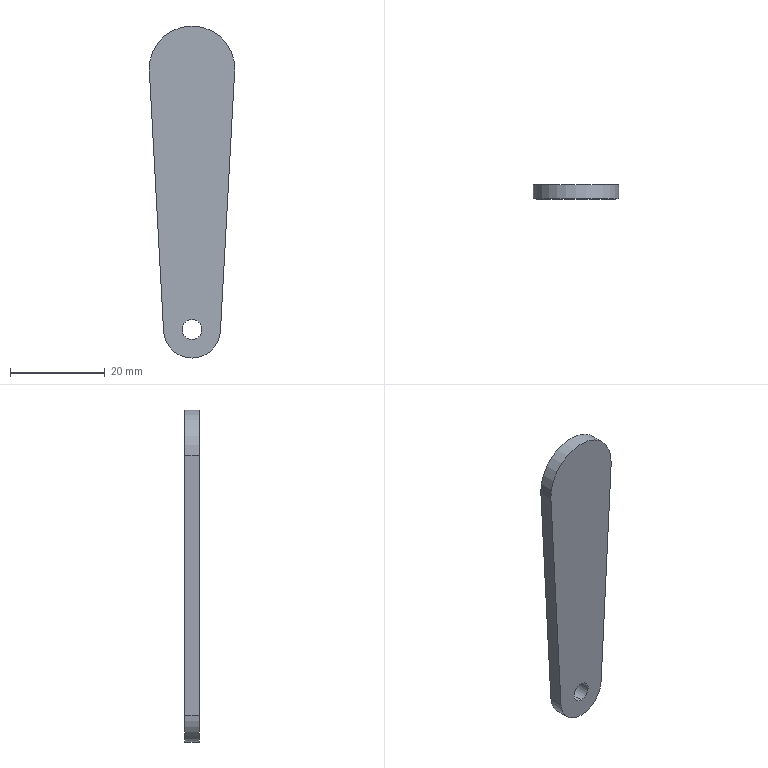Part | STEP file | Handwheel sub-plate | 1 solid | 9 faces | box 18 x 3 x 70 mm | volume 2988 mm3 | cylinder 5 | plane 4 | commonest cylinder face diameters 4.2 x2 12 x2 18 x1
STEP:
#1=CARTESIAN_POINT('',(0.,0.,0.));
#2=DIRECTION('',(0.,0.,1.));
#3=DIRECTION('',(1.,0.,0.));
#4=AXIS2_PLACEMENT_3D('',#1,#2,#3);
#5=CARTESIAN_POINT('',(0.,-1.5,2.1));
#6=VERTEX_POINT('',#5);
#7=CARTESIAN_POINT('',(0.,1.5,2.1));
#8=VERTEX_POINT('',#7);
#9=CARTESIAN_POINT('',(0.,1.5,2.1));
#10=DIRECTION('',(0.,1.,0.));
#11=VECTOR('',#10,1.);
#12=LINE('',#9,#11);
#13=CARTESIAN_POINT('',(0.,1.5,0.));
#14=DIRECTION('',(0.,1.,0.));
#15=DIRECTION('',(0.,0.,1.));
#16=AXIS2_PLACEMENT_3D('',#13,#14,#15);
#17=CYLINDRICAL_SURFACE('',#16,2.1);
#18=CARTESIAN_POINT('',(6.283,0.));
#19=DIRECTION('',(0.,1.));
#20=VECTOR('',#19,1.);
#21=LINE('',#18,#20);
#22=(GEOMETRIC_REPRESENTATION_CONTEXT(2)PARAMETRIC_REPRESENTATION_CONTEXT()REPRESENTATION_CONTEXT('',''));
#23=DEFINITIONAL_REPRESENTATION('',(#21),#22);
#24=PCURVE('',#17,#23);
#25=CARTESIAN_POINT('',(0.,1.5,0.));
#26=DIRECTION('',(0.,1.,0.));
#27=DIRECTION('',(0.,0.,1.));
#28=AXIS2_PLACEMENT_3D('',#25,#26,#27);
#29=CYLINDRICAL_SURFACE('',#28,2.1);
#30=CARTESIAN_POINT('',(0.,0.));
#31=DIRECTION('',(0.,1.));
#32=VECTOR('',#31,1.);
#33=LINE('',#30,#32);
#34=(GEOMETRIC_REPRESENTATION_CONTEXT(2)PARAMETRIC_REPRESENTATION_CONTEXT()REPRESENTATION_CONTEXT('',''));
#35=DEFINITIONAL_REPRESENTATION('',(#33),#34);
#36=PCURVE('',#29,#35);
#37=SURFACE_CURVE('',#12,(#24,#36),.PCURVE_S1.);
#38=EDGE_CURVE('',#6,#8,#37,.T.);
#39=ORIENTED_EDGE('',*,*,#38,.T.);
#40=CARTESIAN_POINT('',(0.,1.5,-2.1));
#41=VERTEX_POINT('',#40);
#42=CARTESIAN_POINT('',(0.,1.5,0.));
#43=DIRECTION('',(0.,1.,0.));
#44=DIRECTION('',(0.,0.,1.));
#45=AXIS2_PLACEMENT_3D('',#42,#43,#44);
#46=CIRCLE('',#45,2.1);
#47=CARTESIAN_POINT('',(0.,0.));
#48=DIRECTION('',(1.,0.));
#49=VECTOR('',#48,1.);
#50=LINE('',#47,#49);
#51=(GEOMETRIC_REPRESENTATION_CONTEXT(2)PARAMETRIC_REPRESENTATION_CONTEXT()REPRESENTATION_CONTEXT('',''));
#52=DEFINITIONAL_REPRESENTATION('',(#50),#51);
#53=PCURVE('',#17,#52);
#54=CARTESIAN_POINT('',(0.,1.5,0.));
#55=DIRECTION('',(0.,1.,0.));
#56=DIRECTION('',(0.,0.,1.));
#57=AXIS2_PLACEMENT_3D('',#54,#55,#56);
#58=PLANE('',#57);
#59=CARTESIAN_POINT('',(0.,0.));
#60=DIRECTION('',(1.,0.));
#61=AXIS2_PLACEMENT_2D('',#59,#60);
#62=CIRCLE('',#61,2.1);
#63=(GEOMETRIC_REPRESENTATION_CONTEXT(2)PARAMETRIC_REPRESENTATION_CONTEXT()REPRESENTATION_CONTEXT('',''));
#64=DEFINITIONAL_REPRESENTATION('',(#62),#63);
#65=PCURVE('',#58,#64);
#66=SURFACE_CURVE('',#46,(#53,#65),.PCURVE_S1.);
#67=EDGE_CURVE('',#41,#8,#66,.T.);
#68=ORIENTED_EDGE('',*,*,#67,.F.);
#69=CARTESIAN_POINT('',(0.,-1.5,-2.1));
#70=VERTEX_POINT('',#69);
#71=CARTESIAN_POINT('',(0.,1.5,-2.1));
#72=DIRECTION('',(0.,1.,0.));
#73=VECTOR('',#72,1.);
#74=LINE('',#71,#73);
#75=CARTESIAN_POINT('',(3.142,0.));
#76=DIRECTION('',(0.,1.));
#77=VECTOR('',#76,1.);
#78=LINE('',#75,#77);
#79=(GEOMETRIC_REPRESENTATION_CONTEXT(2)PARAMETRIC_REPRESENTATION_CONTEXT()REPRESENTATION_CONTEXT('',''));
#80=DEFINITIONAL_REPRESENTATION('',(#78),#79);
#81=PCURVE('',#17,#80);
#82=CARTESIAN_POINT('',(3.142,0.));
#83=DIRECTION('',(0.,1.));
#84=VECTOR('',#83,1.);
#85=LINE('',#82,#84);
#86=(GEOMETRIC_REPRESENTATION_CONTEXT(2)PARAMETRIC_REPRESENTATION_CONTEXT()REPRESENTATION_CONTEXT('',''));
#87=DEFINITIONAL_REPRESENTATION('',(#85),#86);
#88=PCURVE('',#29,#87);
#89=SURFACE_CURVE('',#74,(#81,#88),.PCURVE_S1.);
#90=EDGE_CURVE('',#70,#41,#89,.T.);
#91=ORIENTED_EDGE('',*,*,#90,.F.);
#92=CARTESIAN_POINT('',(0.,-1.5,0.));
#93=DIRECTION('',(0.,1.,0.));
#94=DIRECTION('',(0.,0.,1.));
#95=AXIS2_PLACEMENT_3D('',#92,#93,#94);
#96=CIRCLE('',#95,2.1);
#97=CARTESIAN_POINT('',(0.,-3.));
#98=DIRECTION('',(1.,0.));
#99=VECTOR('',#98,1.);
#100=LINE('',#97,#99);
#101=(GEOMETRIC_REPRESENTATION_CONTEXT(2)PARAMETRIC_REPRESENTATION_CONTEXT()REPRESENTATION_CONTEXT('',''));
#102=DEFINITIONAL_REPRESENTATION('',(#100),#101);
#103=PCURVE('',#17,#102);
#104=CARTESIAN_POINT('',(0.,-1.5,0.));
#105=DIRECTION('',(0.,1.,0.));
#106=DIRECTION('',(0.,0.,1.));
#107=AXIS2_PLACEMENT_3D('',#104,#105,#106);
#108=PLANE('',#107);
#109=CARTESIAN_POINT('',(0.,0.));
#110=DIRECTION('',(1.,0.));
#111=AXIS2_PLACEMENT_2D('',#109,#110);
#112=CIRCLE('',#111,2.1);
#113=(GEOMETRIC_REPRESENTATION_CONTEXT(2)PARAMETRIC_REPRESENTATION_CONTEXT()REPRESENTATION_CONTEXT('',''));
#114=DEFINITIONAL_REPRESENTATION('',(#112),#113);
#115=PCURVE('',#108,#114);
#116=SURFACE_CURVE('',#96,(#103,#115),.PCURVE_S1.);
#117=EDGE_CURVE('',#70,#6,#116,.T.);
#118=ORIENTED_EDGE('',*,*,#117,.T.);
#119=EDGE_LOOP('',(#39,#68,#91,#118));
#120=FACE_BOUND('',#119,.F.);
#121=ADVANCED_FACE('',(#120),#17,.F.);
#122=CARTESIAN_POINT('',(0.,1.5,-6.));
#123=VERTEX_POINT('',#122);
#124=CARTESIAN_POINT('',(-5.991,1.5,-0.3273));
#125=VERTEX_POINT('',#124);
#126=CARTESIAN_POINT('',(0.,1.5,0.));
#127=DIRECTION('',(0.,1.,0.));
#128=DIRECTION('',(0.,0.,1.));
#129=AXIS2_PLACEMENT_3D('',#126,#127,#128);
#130=CIRCLE('',#129,6.);
#131=CARTESIAN_POINT('',(0.,1.5,0.));
#132=DIRECTION('',(0.,-1.,0.));
#133=DIRECTION('',(0.,0.,-1.));
#134=AXIS2_PLACEMENT_3D('',#131,#132,#133);
#135=CYLINDRICAL_SURFACE('',#134,6.);
#136=CARTESIAN_POINT('',(9.425,0.));
#137=DIRECTION('',(-1.,0.));
#138=VECTOR('',#137,1.);
#139=LINE('',#136,#138);
#140=(GEOMETRIC_REPRESENTATION_CONTEXT(2)PARAMETRIC_REPRESENTATION_CONTEXT()REPRESENTATION_CONTEXT('',''));
#141=DEFINITIONAL_REPRESENTATION('',(#139),#140);
#142=PCURVE('',#135,#141);
#143=CARTESIAN_POINT('',(0.,0.));
#144=DIRECTION('',(1.,0.));
#145=AXIS2_PLACEMENT_2D('',#143,#144);
#146=CIRCLE('',#145,6.);
#147=(GEOMETRIC_REPRESENTATION_CONTEXT(2)PARAMETRIC_REPRESENTATION_CONTEXT()REPRESENTATION_CONTEXT('',''));
#148=DEFINITIONAL_REPRESENTATION('',(#146),#147);
#149=PCURVE('',#58,#148);
#150=SURFACE_CURVE('',#130,(#142,#149),.PCURVE_S1.);
#151=EDGE_CURVE('',#123,#125,#150,.T.);
#152=ORIENTED_EDGE('',*,*,#151,.F.);
#153=CARTESIAN_POINT('',(0.,-1.5,-6.));
#154=VERTEX_POINT('',#153);
#155=CARTESIAN_POINT('',(0.,1.5,-6.));
#156=DIRECTION('',(0.,-1.,0.));
#157=VECTOR('',#156,1.);
#158=LINE('',#155,#157);
#159=CARTESIAN_POINT('',(6.283,0.));
#160=DIRECTION('',(0.,1.));
#161=VECTOR('',#160,1.);
#162=LINE('',#159,#161);
#163=(GEOMETRIC_REPRESENTATION_CONTEXT(2)PARAMETRIC_REPRESENTATION_CONTEXT()REPRESENTATION_CONTEXT('',''));
#164=DEFINITIONAL_REPRESENTATION('',(#162),#163);
#165=PCURVE('',#135,#164);
#166=CARTESIAN_POINT('',(0.,1.5,0.));
#167=DIRECTION('',(0.,-1.,0.));
#168=DIRECTION('',(0.,0.,-1.));
#169=AXIS2_PLACEMENT_3D('',#166,#167,#168);
#170=CYLINDRICAL_SURFACE('',#169,6.);
#171=CARTESIAN_POINT('',(0.,0.));
#172=DIRECTION('',(0.,1.));
#173=VECTOR('',#172,1.);
#174=LINE('',#171,#173);
#175=(GEOMETRIC_REPRESENTATION_CONTEXT(2)PARAMETRIC_REPRESENTATION_CONTEXT()REPRESENTATION_CONTEXT('',''));
#176=DEFINITIONAL_REPRESENTATION('',(#174),#175);
#177=PCURVE('',#170,#176);
#178=SURFACE_CURVE('',#158,(#165,#177),.PCURVE_S1.);
#179=EDGE_CURVE('',#123,#154,#178,.T.);
#180=ORIENTED_EDGE('',*,*,#179,.T.);
#181=CARTESIAN_POINT('',(-5.991,-1.5,-0.3273));
#182=VERTEX_POINT('',#181);
#183=CARTESIAN_POINT('',(0.,-1.5,0.));
#184=DIRECTION('',(0.,1.,0.));
#185=DIRECTION('',(0.,0.,1.));
#186=AXIS2_PLACEMENT_3D('',#183,#184,#185);
#187=CIRCLE('',#186,6.);
#188=CARTESIAN_POINT('',(9.425,3.));
#189=DIRECTION('',(-1.,0.));
#190=VECTOR('',#189,1.);
#191=LINE('',#188,#190);
#192=(GEOMETRIC_REPRESENTATION_CONTEXT(2)PARAMETRIC_REPRESENTATION_CONTEXT()REPRESENTATION_CONTEXT('',''));
#193=DEFINITIONAL_REPRESENTATION('',(#191),#192);
#194=PCURVE('',#135,#193);
#195=CARTESIAN_POINT('',(0.,0.));
#196=DIRECTION('',(1.,0.));
#197=AXIS2_PLACEMENT_2D('',#195,#196);
#198=CIRCLE('',#197,6.);
#199=(GEOMETRIC_REPRESENTATION_CONTEXT(2)PARAMETRIC_REPRESENTATION_CONTEXT()REPRESENTATION_CONTEXT('',''));
#200=DEFINITIONAL_REPRESENTATION('',(#198),#199);
#201=PCURVE('',#108,#200);
#202=SURFACE_CURVE('',#187,(#194,#201),.PCURVE_S1.);
#203=EDGE_CURVE('',#154,#182,#202,.T.);
#204=ORIENTED_EDGE('',*,*,#203,.T.);
#205=CARTESIAN_POINT('',(-5.991,1.5,-0.3273));
#206=DIRECTION('',(0.,-1.,0.));
#207=VECTOR('',#206,1.);
#208=LINE('',#205,#207);
#209=CARTESIAN_POINT('',(4.767,0.));
#210=DIRECTION('',(0.,1.));
#211=VECTOR('',#210,1.);
#212=LINE('',#209,#211);
#213=(GEOMETRIC_REPRESENTATION_CONTEXT(2)PARAMETRIC_REPRESENTATION_CONTEXT()REPRESENTATION_CONTEXT('',''));
#214=DEFINITIONAL_REPRESENTATION('',(#212),#213);
#215=PCURVE('',#135,#214);
#216=CARTESIAN_POINT('',(-5.991,1.5,-0.3273));
#217=DIRECTION('',(0.9985,0.,0.05455));
#218=DIRECTION('',(0.05455,0.,-0.9985));
#219=AXIS2_PLACEMENT_3D('',#216,#217,#218);
#220=PLANE('',#219);
#221=CARTESIAN_POINT('',(0.,0.));
#222=DIRECTION('',(0.,-1.));
#223=VECTOR('',#222,1.);
#224=LINE('',#221,#223);
#225=(GEOMETRIC_REPRESENTATION_CONTEXT(2)PARAMETRIC_REPRESENTATION_CONTEXT()REPRESENTATION_CONTEXT('',''));
#226=DEFINITIONAL_REPRESENTATION('',(#224),#225);
#227=PCURVE('',#220,#226);
#228=SURFACE_CURVE('',#208,(#215,#227),.PCURVE_S1.);
#229=EDGE_CURVE('',#125,#182,#228,.T.);
#230=ORIENTED_EDGE('',*,*,#229,.F.);
#231=EDGE_LOOP('',(#152,#180,#204,#230));
#232=FACE_BOUND('',#231,.T.);
#233=ADVANCED_FACE('',(#232),#135,.T.);
#234=ORIENTED_EDGE('',*,*,#179,.F.);
#235=CARTESIAN_POINT('',(5.991,1.5,-0.3273));
#236=VERTEX_POINT('',#235);
#237=CARTESIAN_POINT('',(0.,1.5,0.));
#238=DIRECTION('',(0.,1.,0.));
#239=DIRECTION('',(0.,0.,1.));
#240=AXIS2_PLACEMENT_3D('',#237,#238,#239);
#241=CIRCLE('',#240,6.);
#242=CARTESIAN_POINT('',(3.142,0.));
#243=DIRECTION('',(-1.,0.));
#244=VECTOR('',#243,1.);
#245=LINE('',#242,#244);
#246=(GEOMETRIC_REPRESENTATION_CONTEXT(2)PARAMETRIC_REPRESENTATION_CONTEXT()REPRESENTATION_CONTEXT('',''));
#247=DEFINITIONAL_REPRESENTATION('',(#245),#246);
#248=PCURVE('',#170,#247);
#249=CARTESIAN_POINT('',(0.,0.));
#250=DIRECTION('',(1.,0.));
#251=AXIS2_PLACEMENT_2D('',#249,#250);
#252=CIRCLE('',#251,6.);
#253=(GEOMETRIC_REPRESENTATION_CONTEXT(2)PARAMETRIC_REPRESENTATION_CONTEXT()REPRESENTATION_CONTEXT('',''));
#254=DEFINITIONAL_REPRESENTATION('',(#252),#253);
#255=PCURVE('',#58,#254);
#256=SURFACE_CURVE('',#241,(#248,#255),.PCURVE_S1.);
#257=EDGE_CURVE('',#236,#123,#256,.T.);
#258=ORIENTED_EDGE('',*,*,#257,.F.);
#259=CARTESIAN_POINT('',(5.991,-1.5,-0.3273));
#260=VERTEX_POINT('',#259);
#261=CARTESIAN_POINT('',(5.991,1.5,-0.3273));
#262=DIRECTION('',(0.,-1.,0.));
#263=VECTOR('',#262,1.);
#264=LINE('',#261,#263);
#265=CARTESIAN_POINT('',(1.516,0.));
#266=DIRECTION('',(0.,1.));
#267=VECTOR('',#266,1.);
#268=LINE('',#265,#267);
#269=(GEOMETRIC_REPRESENTATION_CONTEXT(2)PARAMETRIC_REPRESENTATION_CONTEXT()REPRESENTATION_CONTEXT('',''));
#270=DEFINITIONAL_REPRESENTATION('',(#268),#269);
#271=PCURVE('',#170,#270);
#272=CARTESIAN_POINT('',(8.987,1.5,54.509));
#273=DIRECTION('',(-0.9985,0.,0.05455));
#274=DIRECTION('',(0.05455,0.,0.9985));
#275=AXIS2_PLACEMENT_3D('',#272,#273,#274);
#276=PLANE('',#275);
#277=CARTESIAN_POINT('',(-54.918,0.));
#278=DIRECTION('',(0.,-1.));
#279=VECTOR('',#278,1.);
#280=LINE('',#277,#279);
#281=(GEOMETRIC_REPRESENTATION_CONTEXT(2)PARAMETRIC_REPRESENTATION_CONTEXT()REPRESENTATION_CONTEXT('',''));
#282=DEFINITIONAL_REPRESENTATION('',(#280),#281);
#283=PCURVE('',#276,#282);
#284=SURFACE_CURVE('',#264,(#271,#283),.PCURVE_S1.);
#285=EDGE_CURVE('',#236,#260,#284,.T.);
#286=ORIENTED_EDGE('',*,*,#285,.T.);
#287=CARTESIAN_POINT('',(0.,-1.5,0.));
#288=DIRECTION('',(0.,1.,0.));
#289=DIRECTION('',(0.,0.,1.));
#290=AXIS2_PLACEMENT_3D('',#287,#288,#289);
#291=CIRCLE('',#290,6.);
#292=CARTESIAN_POINT('',(3.142,3.));
#293=DIRECTION('',(-1.,0.));
#294=VECTOR('',#293,1.);
#295=LINE('',#292,#294);
#296=(GEOMETRIC_REPRESENTATION_CONTEXT(2)PARAMETRIC_REPRESENTATION_CONTEXT()REPRESENTATION_CONTEXT('',''));
#297=DEFINITIONAL_REPRESENTATION('',(#295),#296);
#298=PCURVE('',#170,#297);
#299=CARTESIAN_POINT('',(0.,0.));
#300=DIRECTION('',(1.,0.));
#301=AXIS2_PLACEMENT_2D('',#299,#300);
#302=CIRCLE('',#301,6.);
#303=(GEOMETRIC_REPRESENTATION_CONTEXT(2)PARAMETRIC_REPRESENTATION_CONTEXT()REPRESENTATION_CONTEXT('',''));
#304=DEFINITIONAL_REPRESENTATION('',(#302),#303);
#305=PCURVE('',#108,#304);
#306=SURFACE_CURVE('',#291,(#298,#305),.PCURVE_S1.);
#307=EDGE_CURVE('',#260,#154,#306,.T.);
#308=ORIENTED_EDGE('',*,*,#307,.T.);
#309=EDGE_LOOP('',(#234,#258,#286,#308));
#310=FACE_BOUND('',#309,.T.);
#311=ADVANCED_FACE('',(#310),#170,.T.);
#312=CARTESIAN_POINT('',(-8.987,-1.5,54.509));
#313=VERTEX_POINT('',#312);
#314=CARTESIAN_POINT('',(-5.991,-1.5,-0.3273));
#315=DIRECTION('',(-0.05455,0.,0.9985));
#316=VECTOR('',#315,1.);
#317=LINE('',#314,#316);
#318=CARTESIAN_POINT('',(0.,-3.));
#319=DIRECTION('',(-1.,0.));
#320=VECTOR('',#319,1.);
#321=LINE('',#318,#320);
#322=(GEOMETRIC_REPRESENTATION_CONTEXT(2)PARAMETRIC_REPRESENTATION_CONTEXT()REPRESENTATION_CONTEXT('',''));
#323=DEFINITIONAL_REPRESENTATION('',(#321),#322);
#324=PCURVE('',#220,#323);
#325=CARTESIAN_POINT('',(-0.3273,-5.991));
#326=DIRECTION('',(0.9985,-0.05455));
#327=VECTOR('',#326,1.);
#328=LINE('',#325,#327);
#329=(GEOMETRIC_REPRESENTATION_CONTEXT(2)PARAMETRIC_REPRESENTATION_CONTEXT()REPRESENTATION_CONTEXT('',''));
#330=DEFINITIONAL_REPRESENTATION('',(#328),#329);
#331=PCURVE('',#108,#330);
#332=SURFACE_CURVE('',#317,(#324,#331),.PCURVE_S1.);
#333=EDGE_CURVE('',#182,#313,#332,.T.);
#334=ORIENTED_EDGE('',*,*,#333,.T.);
#335=CARTESIAN_POINT('',(-8.987,1.5,54.509));
#336=VERTEX_POINT('',#335);
#337=CARTESIAN_POINT('',(-8.987,1.5,54.509));
#338=DIRECTION('',(0.,-1.,0.));
#339=VECTOR('',#338,1.);
#340=LINE('',#337,#339);
#341=CARTESIAN_POINT('',(-54.918,0.));
#342=DIRECTION('',(0.,-1.));
#343=VECTOR('',#342,1.);
#344=LINE('',#341,#343);
#345=(GEOMETRIC_REPRESENTATION_CONTEXT(2)PARAMETRIC_REPRESENTATION_CONTEXT()REPRESENTATION_CONTEXT('',''));
#346=DEFINITIONAL_REPRESENTATION('',(#344),#345);
#347=PCURVE('',#220,#346);
#348=CARTESIAN_POINT('',(0.,1.5,55.));
#349=DIRECTION('',(0.,-1.,0.));
#350=DIRECTION('',(0.,0.,-1.));
#351=AXIS2_PLACEMENT_3D('',#348,#349,#350);
#352=CYLINDRICAL_SURFACE('',#351,9.);
#353=CARTESIAN_POINT('',(4.767,0.));
#354=DIRECTION('',(0.,1.));
#355=VECTOR('',#354,1.);
#356=LINE('',#353,#355);
#357=(GEOMETRIC_REPRESENTATION_CONTEXT(2)PARAMETRIC_REPRESENTATION_CONTEXT()REPRESENTATION_CONTEXT('',''));
#358=DEFINITIONAL_REPRESENTATION('',(#356),#357);
#359=PCURVE('',#352,#358);
#360=SURFACE_CURVE('',#340,(#347,#359),.PCURVE_S1.);
#361=EDGE_CURVE('',#336,#313,#360,.T.);
#362=ORIENTED_EDGE('',*,*,#361,.F.);
#363=CARTESIAN_POINT('',(-5.991,1.5,-0.3273));
#364=DIRECTION('',(-0.05455,0.,0.9985));
#365=VECTOR('',#364,1.);
#366=LINE('',#363,#365);
#367=CARTESIAN_POINT('',(0.,0.));
#368=DIRECTION('',(-1.,0.));
#369=VECTOR('',#368,1.);
#370=LINE('',#367,#369);
#371=(GEOMETRIC_REPRESENTATION_CONTEXT(2)PARAMETRIC_REPRESENTATION_CONTEXT()REPRESENTATION_CONTEXT('',''));
#372=DEFINITIONAL_REPRESENTATION('',(#370),#371);
#373=PCURVE('',#220,#372);
#374=CARTESIAN_POINT('',(-0.3273,-5.991));
#375=DIRECTION('',(0.9985,-0.05455));
#376=VECTOR('',#375,1.);
#377=LINE('',#374,#376);
#378=(GEOMETRIC_REPRESENTATION_CONTEXT(2)PARAMETRIC_REPRESENTATION_CONTEXT()REPRESENTATION_CONTEXT('',''));
#379=DEFINITIONAL_REPRESENTATION('',(#377),#378);
#380=PCURVE('',#58,#379);
#381=SURFACE_CURVE('',#366,(#373,#380),.PCURVE_S1.);
#382=EDGE_CURVE('',#125,#336,#381,.T.);
#383=ORIENTED_EDGE('',*,*,#382,.F.);
#384=ORIENTED_EDGE('',*,*,#229,.T.);
#385=EDGE_LOOP('',(#334,#362,#383,#384));
#386=FACE_BOUND('',#385,.T.);
#387=ADVANCED_FACE('',(#386),#220,.F.);
#388=CARTESIAN_POINT('',(8.987,-1.5,54.509));
#389=VERTEX_POINT('',#388);
#390=CARTESIAN_POINT('',(0.,-1.5,55.));
#391=DIRECTION('',(0.,1.,0.));
#392=DIRECTION('',(0.,0.,1.));
#393=AXIS2_PLACEMENT_3D('',#390,#391,#392);
#394=CIRCLE('',#393,9.);
#395=CARTESIAN_POINT('',(9.425,3.));
#396=DIRECTION('',(-1.,0.));
#397=VECTOR('',#396,1.);
#398=LINE('',#395,#397);
#399=(GEOMETRIC_REPRESENTATION_CONTEXT(2)PARAMETRIC_REPRESENTATION_CONTEXT()REPRESENTATION_CONTEXT('',''));
#400=DEFINITIONAL_REPRESENTATION('',(#398),#399);
#401=PCURVE('',#352,#400);
#402=CARTESIAN_POINT('',(55.,0.));
#403=DIRECTION('',(1.,0.));
#404=AXIS2_PLACEMENT_2D('',#402,#403);
#405=CIRCLE('',#404,9.);
#406=(GEOMETRIC_REPRESENTATION_CONTEXT(2)PARAMETRIC_REPRESENTATION_CONTEXT()REPRESENTATION_CONTEXT('',''));
#407=DEFINITIONAL_REPRESENTATION('',(#405),#406);
#408=PCURVE('',#108,#407);
#409=SURFACE_CURVE('',#394,(#401,#408),.PCURVE_S1.);
#410=EDGE_CURVE('',#313,#389,#409,.T.);
#411=ORIENTED_EDGE('',*,*,#410,.T.);
#412=CARTESIAN_POINT('',(8.987,1.5,54.509));
#413=VERTEX_POINT('',#412);
#414=CARTESIAN_POINT('',(8.987,1.5,54.509));
#415=DIRECTION('',(0.,-1.,0.));
#416=VECTOR('',#415,1.);
#417=LINE('',#414,#416);
#418=CARTESIAN_POINT('',(1.516,0.));
#419=DIRECTION('',(0.,1.));
#420=VECTOR('',#419,1.);
#421=LINE('',#418,#420);
#422=(GEOMETRIC_REPRESENTATION_CONTEXT(2)PARAMETRIC_REPRESENTATION_CONTEXT()REPRESENTATION_CONTEXT('',''));
#423=DEFINITIONAL_REPRESENTATION('',(#421),#422);
#424=PCURVE('',#352,#423);
#425=CARTESIAN_POINT('',(0.,0.));
#426=DIRECTION('',(0.,-1.));
#427=VECTOR('',#426,1.);
#428=LINE('',#425,#427);
#429=(GEOMETRIC_REPRESENTATION_CONTEXT(2)PARAMETRIC_REPRESENTATION_CONTEXT()REPRESENTATION_CONTEXT('',''));
#430=DEFINITIONAL_REPRESENTATION('',(#428),#429);
#431=PCURVE('',#276,#430);
#432=SURFACE_CURVE('',#417,(#424,#431),.PCURVE_S1.);
#433=EDGE_CURVE('',#413,#389,#432,.T.);
#434=ORIENTED_EDGE('',*,*,#433,.F.);
#435=CARTESIAN_POINT('',(0.,1.5,55.));
#436=DIRECTION('',(0.,1.,0.));
#437=DIRECTION('',(0.,0.,1.));
#438=AXIS2_PLACEMENT_3D('',#435,#436,#437);
#439=CIRCLE('',#438,9.);
#440=CARTESIAN_POINT('',(9.425,0.));
#441=DIRECTION('',(-1.,0.));
#442=VECTOR('',#441,1.);
#443=LINE('',#440,#442);
#444=(GEOMETRIC_REPRESENTATION_CONTEXT(2)PARAMETRIC_REPRESENTATION_CONTEXT()REPRESENTATION_CONTEXT('',''));
#445=DEFINITIONAL_REPRESENTATION('',(#443),#444);
#446=PCURVE('',#352,#445);
#447=CARTESIAN_POINT('',(55.,0.));
#448=DIRECTION('',(1.,0.));
#449=AXIS2_PLACEMENT_2D('',#447,#448);
#450=CIRCLE('',#449,9.);
#451=(GEOMETRIC_REPRESENTATION_CONTEXT(2)PARAMETRIC_REPRESENTATION_CONTEXT()REPRESENTATION_CONTEXT('',''));
#452=DEFINITIONAL_REPRESENTATION('',(#450),#451);
#453=PCURVE('',#58,#452);
#454=SURFACE_CURVE('',#439,(#446,#453),.PCURVE_S1.);
#455=EDGE_CURVE('',#336,#413,#454,.T.);
#456=ORIENTED_EDGE('',*,*,#455,.F.);
#457=ORIENTED_EDGE('',*,*,#361,.T.);
#458=EDGE_LOOP('',(#411,#434,#456,#457));
#459=FACE_BOUND('',#458,.T.);
#460=ADVANCED_FACE('',(#459),#352,.T.);
#461=CARTESIAN_POINT('',(8.987,-1.5,54.509));
#462=DIRECTION('',(-0.05455,0.,-0.9985));
#463=VECTOR('',#462,1.);
#464=LINE('',#461,#463);
#465=CARTESIAN_POINT('',(0.,-3.));
#466=DIRECTION('',(-1.,0.));
#467=VECTOR('',#466,1.);
#468=LINE('',#465,#467);
#469=(GEOMETRIC_REPRESENTATION_CONTEXT(2)PARAMETRIC_REPRESENTATION_CONTEXT()REPRESENTATION_CONTEXT('',''));
#470=DEFINITIONAL_REPRESENTATION('',(#468),#469);
#471=PCURVE('',#276,#470);
#472=CARTESIAN_POINT('',(54.509,8.987));
#473=DIRECTION('',(-0.9985,-0.05455));
#474=VECTOR('',#473,1.);
#475=LINE('',#472,#474);
#476=(GEOMETRIC_REPRESENTATION_CONTEXT(2)PARAMETRIC_REPRESENTATION_CONTEXT()REPRESENTATION_CONTEXT('',''));
#477=DEFINITIONAL_REPRESENTATION('',(#475),#476);
#478=PCURVE('',#108,#477);
#479=SURFACE_CURVE('',#464,(#471,#478),.PCURVE_S1.);
#480=EDGE_CURVE('',#389,#260,#479,.T.);
#481=ORIENTED_EDGE('',*,*,#480,.T.);
#482=ORIENTED_EDGE('',*,*,#285,.F.);
#483=CARTESIAN_POINT('',(8.987,1.5,54.509));
#484=DIRECTION('',(-0.05455,0.,-0.9985));
#485=VECTOR('',#484,1.);
#486=LINE('',#483,#485);
#487=CARTESIAN_POINT('',(0.,0.));
#488=DIRECTION('',(-1.,0.));
#489=VECTOR('',#488,1.);
#490=LINE('',#487,#489);
#491=(GEOMETRIC_REPRESENTATION_CONTEXT(2)PARAMETRIC_REPRESENTATION_CONTEXT()REPRESENTATION_CONTEXT('',''));
#492=DEFINITIONAL_REPRESENTATION('',(#490),#491);
#493=PCURVE('',#276,#492);
#494=CARTESIAN_POINT('',(54.509,8.987));
#495=DIRECTION('',(-0.9985,-0.05455));
#496=VECTOR('',#495,1.);
#497=LINE('',#494,#496);
#498=(GEOMETRIC_REPRESENTATION_CONTEXT(2)PARAMETRIC_REPRESENTATION_CONTEXT()REPRESENTATION_CONTEXT('',''));
#499=DEFINITIONAL_REPRESENTATION('',(#497),#498);
#500=PCURVE('',#58,#499);
#501=SURFACE_CURVE('',#486,(#493,#500),.PCURVE_S1.);
#502=EDGE_CURVE('',#413,#236,#501,.T.);
#503=ORIENTED_EDGE('',*,*,#502,.F.);
#504=ORIENTED_EDGE('',*,*,#433,.T.);
#505=EDGE_LOOP('',(#481,#482,#503,#504));
#506=FACE_BOUND('',#505,.T.);
#507=ADVANCED_FACE('',(#506),#276,.F.);
#508=CARTESIAN_POINT('',(0.,1.5,0.));
#509=DIRECTION('',(0.,1.,0.));
#510=DIRECTION('',(0.,0.,1.));
#511=AXIS2_PLACEMENT_3D('',#508,#509,#510);
#512=CIRCLE('',#511,2.1);
#513=CARTESIAN_POINT('',(0.,0.));
#514=DIRECTION('',(1.,0.));
#515=AXIS2_PLACEMENT_2D('',#513,#514);
#516=CIRCLE('',#515,2.1);
#517=(GEOMETRIC_REPRESENTATION_CONTEXT(2)PARAMETRIC_REPRESENTATION_CONTEXT()REPRESENTATION_CONTEXT('',''));
#518=DEFINITIONAL_REPRESENTATION('',(#516),#517);
#519=PCURVE('',#58,#518);
#520=CARTESIAN_POINT('',(0.,0.));
#521=DIRECTION('',(1.,0.));
#522=VECTOR('',#521,1.);
#523=LINE('',#520,#522);
#524=(GEOMETRIC_REPRESENTATION_CONTEXT(2)PARAMETRIC_REPRESENTATION_CONTEXT()REPRESENTATION_CONTEXT('',''));
#525=DEFINITIONAL_REPRESENTATION('',(#523),#524);
#526=PCURVE('',#29,#525);
#527=SURFACE_CURVE('',#512,(#519,#526),.PCURVE_S1.);
#528=EDGE_CURVE('',#8,#41,#527,.T.);
#529=ORIENTED_EDGE('',*,*,#528,.F.);
#530=ORIENTED_EDGE('',*,*,#67,.F.);
#531=EDGE_LOOP('',(#529,#530));
#532=FACE_BOUND('',#531,.T.);
#533=ORIENTED_EDGE('',*,*,#257,.T.);
#534=ORIENTED_EDGE('',*,*,#151,.T.);
#535=ORIENTED_EDGE('',*,*,#382,.T.);
#536=ORIENTED_EDGE('',*,*,#455,.T.);
#537=ORIENTED_EDGE('',*,*,#502,.T.);
#538=EDGE_LOOP('',(#533,#534,#535,#536,#537));
#539=FACE_BOUND('',#538,.T.);
#540=ADVANCED_FACE('',(#532,#539),#58,.T.);
#541=CARTESIAN_POINT('',(0.,-1.5,0.));
#542=DIRECTION('',(0.,1.,0.));
#543=DIRECTION('',(0.,0.,1.));
#544=AXIS2_PLACEMENT_3D('',#541,#542,#543);
#545=CIRCLE('',#544,2.1);
#546=CARTESIAN_POINT('',(0.,0.));
#547=DIRECTION('',(1.,0.));
#548=AXIS2_PLACEMENT_2D('',#546,#547);
#549=CIRCLE('',#548,2.1);
#550=(GEOMETRIC_REPRESENTATION_CONTEXT(2)PARAMETRIC_REPRESENTATION_CONTEXT()REPRESENTATION_CONTEXT('',''));
#551=DEFINITIONAL_REPRESENTATION('',(#549),#550);
#552=PCURVE('',#108,#551);
#553=CARTESIAN_POINT('',(0.,-3.));
#554=DIRECTION('',(1.,0.));
#555=VECTOR('',#554,1.);
#556=LINE('',#553,#555);
#557=(GEOMETRIC_REPRESENTATION_CONTEXT(2)PARAMETRIC_REPRESENTATION_CONTEXT()REPRESENTATION_CONTEXT('',''));
#558=DEFINITIONAL_REPRESENTATION('',(#556),#557);
#559=PCURVE('',#29,#558);
#560=SURFACE_CURVE('',#545,(#552,#559),.PCURVE_S1.);
#561=EDGE_CURVE('',#6,#70,#560,.T.);
#562=ORIENTED_EDGE('',*,*,#561,.T.);
#563=ORIENTED_EDGE('',*,*,#117,.T.);
#564=EDGE_LOOP('',(#562,#563));
#565=FACE_BOUND('',#564,.T.);
#566=ORIENTED_EDGE('',*,*,#307,.F.);
#567=ORIENTED_EDGE('',*,*,#480,.F.);
#568=ORIENTED_EDGE('',*,*,#410,.F.);
#569=ORIENTED_EDGE('',*,*,#333,.F.);
#570=ORIENTED_EDGE('',*,*,#203,.F.);
#571=EDGE_LOOP('',(#566,#567,#568,#569,#570));
#572=FACE_BOUND('',#571,.T.);
#573=ADVANCED_FACE('',(#565,#572),#108,.F.);
#574=ORIENTED_EDGE('',*,*,#528,.F.);
#575=ORIENTED_EDGE('',*,*,#38,.F.);
#576=ORIENTED_EDGE('',*,*,#561,.T.);
#577=ORIENTED_EDGE('',*,*,#90,.T.);
#578=EDGE_LOOP('',(#574,#575,#576,#577));
#579=FACE_BOUND('',#578,.F.);
#580=ADVANCED_FACE('',(#579),#29,.F.);
#581=CLOSED_SHELL('',(#121,#233,#311,#387,#460,#507,#540,#573,#580));
#582=MANIFOLD_SOLID_BREP('',#581);
#583=(LENGTH_UNIT()NAMED_UNIT(*)SI_UNIT(.MILLI.,.METRE.));
#584=UNCERTAINTY_MEASURE_WITH_UNIT(LENGTH_MEASURE(0.0000001),#583,'','');
#585=(NAMED_UNIT(*)PLANE_ANGLE_UNIT()SI_UNIT($,.RADIAN.));
#586=(NAMED_UNIT(*)SI_UNIT($,.STERADIAN.)SOLID_ANGLE_UNIT());
#587=(GEOMETRIC_REPRESENTATION_CONTEXT(3)GLOBAL_UNCERTAINTY_ASSIGNED_CONTEXT((#584))GLOBAL_UNIT_ASSIGNED_CONTEXT((#583,#585,#586))REPRESENTATION_CONTEXT('',''));
#588=ADVANCED_BREP_SHAPE_REPRESENTATION('',(#4,#582),#587);